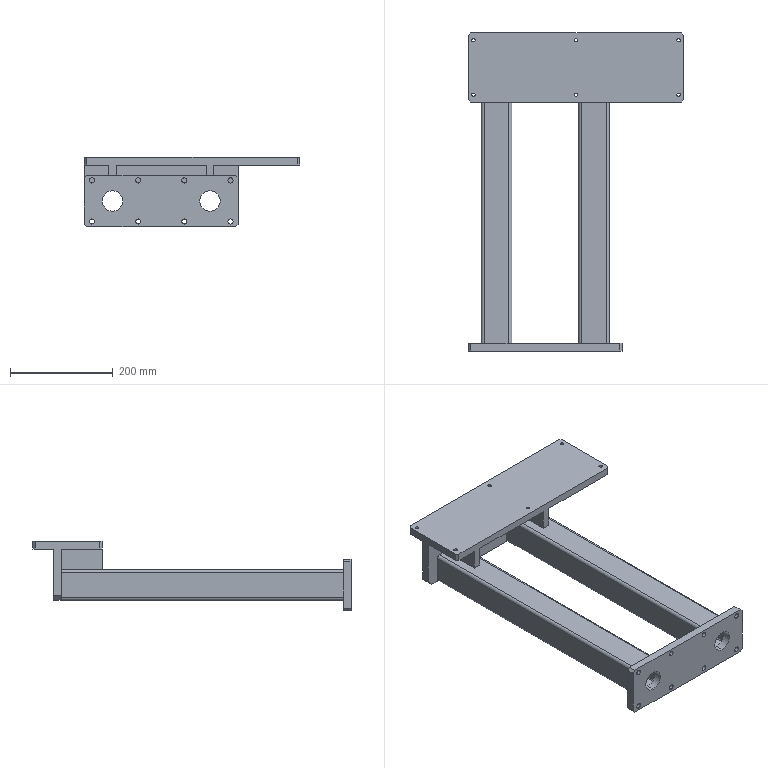Part | SolidWorks | features ICE 7, Chamfer 3, LPattern 2, Extrusion 1, HoleWzd 1 | 1 solid | 138 faces | box 420 x 620 x 135 mm | volume 2694672 mm3 | cylinder 72 | plane 66 | commonest cylinder face diameters 10 x24 6.6 x12 11 x12 4 x8 12 x8 40 x8